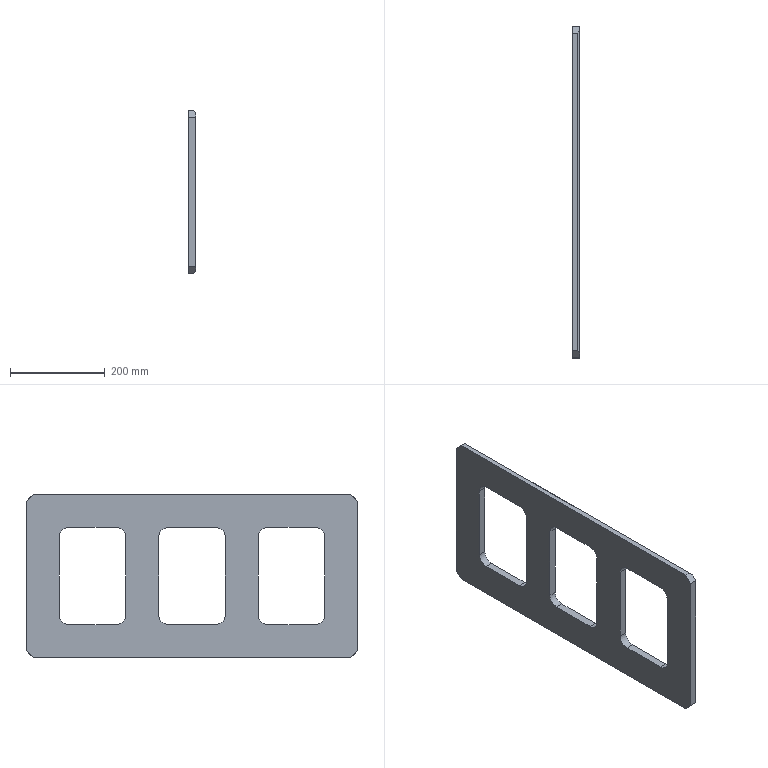Part | SolidWorks | features Chamfer 2, FlatPattern 1, ICE 1, LPattern 1, SMBaseFlange 1, SheetMetal 1 | 1 solid | 36 faces | box 16 x 700 x 345 mm | volume 2478848 mm3 | plane 24 | cylinder 12 | commonest cylinder face diameters 40 x12
STEP:
#1=CARTESIAN_POINT('',(-16.,15.,0.));
#2=VERTEX_POINT('',#1);
#3=CARTESIAN_POINT('',(-5.,15.,0.));
#4=VERTEX_POINT('',#3);
#5=CARTESIAN_POINT('',(-16.,15.,0.));
#6=DIRECTION('',(1.,0.,0.));
#7=VECTOR('',#6,1000.);
#8=LINE('',#5,#7);
#9=EDGE_CURVE('',#2,#4,#8,.T.);
#10=ORIENTED_EDGE('',*,*,#9,.T.);
#11=CARTESIAN_POINT('',(-5.,685.,0.));
#12=VERTEX_POINT('',#11);
#13=CARTESIAN_POINT('',(-5.,685.,0.));
#14=DIRECTION('',(0.,1.,0.));
#15=VECTOR('',#14,1000.);
#16=LINE('',#13,#15);
#17=EDGE_CURVE('',#4,#12,#16,.T.);
#18=ORIENTED_EDGE('',*,*,#17,.T.);
#19=CARTESIAN_POINT('',(-16.,685.,0.));
#20=VERTEX_POINT('',#19);
#21=CARTESIAN_POINT('',(-16.,685.,0.));
#22=DIRECTION('',(-1.,0.,0.));
#23=VECTOR('',#22,1000.);
#24=LINE('',#21,#23);
#25=EDGE_CURVE('',#12,#20,#24,.T.);
#26=ORIENTED_EDGE('',*,*,#25,.T.);
#27=CARTESIAN_POINT('',(-16.,0.,0.));
#28=DIRECTION('',(0.,-1.,0.));
#29=VECTOR('',#28,1000.);
#30=LINE('',#27,#29);
#31=EDGE_CURVE('',#20,#2,#30,.T.);
#32=ORIENTED_EDGE('',*,*,#31,.T.);
#33=EDGE_LOOP('',(#10,#18,#26,#32));
#34=FACE_OUTER_BOUND('',#33,.T.);
#35=CARTESIAN_POINT('',(-16.,0.,0.));
#36=DIRECTION('',(0.,0.,1.));
#37=DIRECTION('',(1.,0.,0.));
#38=AXIS2_PLACEMENT_3D('',#35,#36,#37);
#39=PLANE('',#38);
#40=ADVANCED_FACE('',(#34),#39,.T.);
#41=CARTESIAN_POINT('',(0.,700.,-330.));
#42=VERTEX_POINT('',#41);
#43=CARTESIAN_POINT('',(0.,700.,-15.));
#44=VERTEX_POINT('',#43);
#45=CARTESIAN_POINT('',(0.,700.,0.));
#46=DIRECTION('',(0.,0.,1.));
#47=VECTOR('',#46,1000.);
#48=LINE('',#45,#47);
#49=EDGE_CURVE('',#42,#44,#48,.T.);
#50=ORIENTED_EDGE('',*,*,#49,.F.);
#51=CARTESIAN_POINT('',(-16.,700.,-330.));
#52=VERTEX_POINT('',#51);
#53=CARTESIAN_POINT('',(-16.,700.,-330.));
#54=DIRECTION('',(-1.,0.,0.));
#55=VECTOR('',#54,1000.);
#56=LINE('',#53,#55);
#57=EDGE_CURVE('',#42,#52,#56,.T.);
#58=ORIENTED_EDGE('',*,*,#57,.T.);
#59=CARTESIAN_POINT('',(-16.,700.,-15.));
#60=VERTEX_POINT('',#59);
#61=CARTESIAN_POINT('',(-16.,700.,0.));
#62=DIRECTION('',(0.,0.,1.));
#63=VECTOR('',#62,1000.);
#64=LINE('',#61,#63);
#65=EDGE_CURVE('',#52,#60,#64,.T.);
#66=ORIENTED_EDGE('',*,*,#65,.T.);
#67=CARTESIAN_POINT('',(-16.,700.,-15.));
#68=DIRECTION('',(1.,0.,0.));
#69=VECTOR('',#68,1000.);
#70=LINE('',#67,#69);
#71=EDGE_CURVE('',#60,#44,#70,.T.);
#72=ORIENTED_EDGE('',*,*,#71,.T.);
#73=EDGE_LOOP('',(#50,#58,#66,#72));
#74=FACE_OUTER_BOUND('',#73,.T.);
#75=CARTESIAN_POINT('',(-16.,700.,0.));
#76=DIRECTION('',(0.,1.,0.));
#77=DIRECTION('',(0.,0.,1.));
#78=AXIS2_PLACEMENT_3D('',#75,#76,#77);
#79=PLANE('',#78);
#80=ADVANCED_FACE('',(#74),#79,.T.);
#81=CARTESIAN_POINT('',(-16.,685.,-345.));
#82=VERTEX_POINT('',#81);
#83=CARTESIAN_POINT('',(-5.,685.,-345.));
#84=VERTEX_POINT('',#83);
#85=CARTESIAN_POINT('',(-16.,685.,-345.));
#86=DIRECTION('',(1.,0.,0.));
#87=VECTOR('',#86,1000.);
#88=LINE('',#85,#87);
#89=EDGE_CURVE('',#82,#84,#88,.T.);
#90=ORIENTED_EDGE('',*,*,#89,.T.);
#91=CARTESIAN_POINT('',(-5.,15.,-345.));
#92=VERTEX_POINT('',#91);
#93=CARTESIAN_POINT('',(-5.,15.,-345.));
#94=DIRECTION('',(0.,-1.,0.));
#95=VECTOR('',#94,1000.);
#96=LINE('',#93,#95);
#97=EDGE_CURVE('',#84,#92,#96,.T.);
#98=ORIENTED_EDGE('',*,*,#97,.T.);
#99=CARTESIAN_POINT('',(-16.,15.,-345.));
#100=VERTEX_POINT('',#99);
#101=CARTESIAN_POINT('',(-16.,15.,-345.));
#102=DIRECTION('',(-1.,0.,0.));
#103=VECTOR('',#102,1000.);
#104=LINE('',#101,#103);
#105=EDGE_CURVE('',#92,#100,#104,.T.);
#106=ORIENTED_EDGE('',*,*,#105,.T.);
#107=CARTESIAN_POINT('',(-16.,0.,-345.));
#108=DIRECTION('',(0.,1.,0.));
#109=VECTOR('',#108,1000.);
#110=LINE('',#107,#109);
#111=EDGE_CURVE('',#100,#82,#110,.T.);
#112=ORIENTED_EDGE('',*,*,#111,.T.);
#113=EDGE_LOOP('',(#90,#98,#106,#112));
#114=FACE_OUTER_BOUND('',#113,.T.);
#115=CARTESIAN_POINT('',(-16.,0.,-345.));
#116=DIRECTION('',(0.,0.,-1.));
#117=DIRECTION('',(-1.,0.,0.));
#118=AXIS2_PLACEMENT_3D('',#115,#116,#117);
#119=PLANE('',#118);
#120=ADVANCED_FACE('',(#114),#119,.T.);
#121=CARTESIAN_POINT('',(-16.,0.,-15.));
#122=VERTEX_POINT('',#121);
#123=CARTESIAN_POINT('',(-16.,0.,-330.));
#124=VERTEX_POINT('',#123);
#125=CARTESIAN_POINT('',(-16.,0.,0.));
#126=DIRECTION('',(0.,0.,-1.));
#127=VECTOR('',#126,1000.);
#128=LINE('',#125,#127);
#129=EDGE_CURVE('',#122,#124,#128,.T.);
#130=ORIENTED_EDGE('',*,*,#129,.T.);
#131=CARTESIAN_POINT('',(0.,0.,-330.));
#132=VERTEX_POINT('',#131);
#133=CARTESIAN_POINT('',(-16.,0.,-330.));
#134=DIRECTION('',(1.,0.,0.));
#135=VECTOR('',#134,1000.);
#136=LINE('',#133,#135);
#137=EDGE_CURVE('',#124,#132,#136,.T.);
#138=ORIENTED_EDGE('',*,*,#137,.T.);
#139=CARTESIAN_POINT('',(0.,0.,-15.));
#140=VERTEX_POINT('',#139);
#141=CARTESIAN_POINT('',(0.,0.,0.));
#142=DIRECTION('',(0.,0.,-1.));
#143=VECTOR('',#142,1000.);
#144=LINE('',#141,#143);
#145=EDGE_CURVE('',#140,#132,#144,.T.);
#146=ORIENTED_EDGE('',*,*,#145,.F.);
#147=CARTESIAN_POINT('',(-16.,0.,-15.));
#148=DIRECTION('',(-1.,0.,0.));
#149=VECTOR('',#148,1000.);
#150=LINE('',#147,#149);
#151=EDGE_CURVE('',#140,#122,#150,.T.);
#152=ORIENTED_EDGE('',*,*,#151,.T.);
#153=EDGE_LOOP('',(#130,#138,#146,#152));
#154=FACE_OUTER_BOUND('',#153,.T.);
#155=CARTESIAN_POINT('',(-16.,0.,0.));
#156=DIRECTION('',(0.,-1.,0.));
#157=DIRECTION('',(0.,0.,-1.));
#158=AXIS2_PLACEMENT_3D('',#155,#156,#157);
#159=PLANE('',#158);
#160=ADVANCED_FACE('',(#154),#159,.T.);
#161=CARTESIAN_POINT('',(-16.,300.,-70.));
#162=VERTEX_POINT('',#161);
#163=CARTESIAN_POINT('',(-16.,280.,-90.));
#164=VERTEX_POINT('',#163);
#165=CARTESIAN_POINT('',(-16.,300.,-90.));
#166=DIRECTION('',(1.,0.,0.));
#167=DIRECTION('',(0.,0.,1.));
#168=AXIS2_PLACEMENT_3D('',#165,#166,#167);
#169=CIRCLE('',#168,20.);
#170=EDGE_CURVE('',#162,#164,#169,.T.);
#171=ORIENTED_EDGE('',*,*,#170,.T.);
#172=CARTESIAN_POINT('',(-16.,280.,-255.));
#173=VERTEX_POINT('',#172);
#174=CARTESIAN_POINT('',(-16.,280.,-90.));
#175=DIRECTION('',(0.,0.,-1.));
#176=VECTOR('',#175,1000.);
#177=LINE('',#174,#176);
#178=EDGE_CURVE('',#164,#173,#177,.T.);
#179=ORIENTED_EDGE('',*,*,#178,.T.);
#180=CARTESIAN_POINT('',(-16.,300.,-275.));
#181=VERTEX_POINT('',#180);
#182=CARTESIAN_POINT('',(-16.,300.,-255.));
#183=DIRECTION('',(1.,0.,0.));
#184=DIRECTION('',(0.,0.,-1.));
#185=AXIS2_PLACEMENT_3D('',#182,#183,#184);
#186=CIRCLE('',#185,20.);
#187=EDGE_CURVE('',#173,#181,#186,.T.);
#188=ORIENTED_EDGE('',*,*,#187,.T.);
#189=CARTESIAN_POINT('',(-16.,400.,-275.));
#190=VERTEX_POINT('',#189);
#191=CARTESIAN_POINT('',(-16.,400.,-275.));
#192=DIRECTION('',(0.,1.,0.));
#193=VECTOR('',#192,1000.);
#194=LINE('',#191,#193);
#195=EDGE_CURVE('',#181,#190,#194,.T.);
#196=ORIENTED_EDGE('',*,*,#195,.T.);
#197=CARTESIAN_POINT('',(-16.,420.,-255.));
#198=VERTEX_POINT('',#197);
#199=CARTESIAN_POINT('',(-16.,400.,-255.));
#200=DIRECTION('',(1.,0.,0.));
#201=DIRECTION('',(0.,0.,-1.));
#202=AXIS2_PLACEMENT_3D('',#199,#200,#201);
#203=CIRCLE('',#202,20.);
#204=EDGE_CURVE('',#190,#198,#203,.T.);
#205=ORIENTED_EDGE('',*,*,#204,.T.);
#206=CARTESIAN_POINT('',(-16.,420.,-90.));
#207=VERTEX_POINT('',#206);
#208=CARTESIAN_POINT('',(-16.,420.,-90.));
#209=DIRECTION('',(0.,0.,1.));
#210=VECTOR('',#209,1000.);
#211=LINE('',#208,#210);
#212=EDGE_CURVE('',#198,#207,#211,.T.);
#213=ORIENTED_EDGE('',*,*,#212,.T.);
#214=CARTESIAN_POINT('',(-16.,400.,-70.));
#215=VERTEX_POINT('',#214);
#216=CARTESIAN_POINT('',(-16.,400.,-90.));
#217=DIRECTION('',(1.,0.,0.));
#218=DIRECTION('',(0.,0.,-1.));
#219=AXIS2_PLACEMENT_3D('',#216,#217,#218);
#220=CIRCLE('',#219,20.);
#221=EDGE_CURVE('',#207,#215,#220,.T.);
#222=ORIENTED_EDGE('',*,*,#221,.T.);
#223=CARTESIAN_POINT('',(-16.,400.,-70.));
#224=DIRECTION('',(0.,-1.,0.));
#225=VECTOR('',#224,1000.);
#226=LINE('',#223,#225);
#227=EDGE_CURVE('',#215,#162,#226,.T.);
#228=ORIENTED_EDGE('',*,*,#227,.T.);
#229=EDGE_LOOP('',(#171,#179,#188,#196,#205,#213,#222,#228));
#230=FACE_BOUND('',#229,.T.);
#231=CARTESIAN_POINT('',(-16.,510.,-70.));
#232=VERTEX_POINT('',#231);
#233=CARTESIAN_POINT('',(-16.,490.,-90.));
#234=VERTEX_POINT('',#233);
#235=CARTESIAN_POINT('',(-16.,510.,-90.));
#236=DIRECTION('',(1.,0.,0.));
#237=DIRECTION('',(0.,0.,1.));
#238=AXIS2_PLACEMENT_3D('',#235,#236,#237);
#239=CIRCLE('',#238,20.);
#240=EDGE_CURVE('',#232,#234,#239,.T.);
#241=ORIENTED_EDGE('',*,*,#240,.T.);
#242=CARTESIAN_POINT('',(-16.,490.,-255.));
#243=VERTEX_POINT('',#242);
#244=CARTESIAN_POINT('',(-16.,490.,-90.));
#245=DIRECTION('',(0.,0.,-1.));
#246=VECTOR('',#245,1000.);
#247=LINE('',#244,#246);
#248=EDGE_CURVE('',#234,#243,#247,.T.);
#249=ORIENTED_EDGE('',*,*,#248,.T.);
#250=CARTESIAN_POINT('',(-16.,510.,-275.));
#251=VERTEX_POINT('',#250);
#252=CARTESIAN_POINT('',(-16.,510.,-255.));
#253=DIRECTION('',(1.,0.,0.));
#254=DIRECTION('',(0.,0.,-1.));
#255=AXIS2_PLACEMENT_3D('',#252,#253,#254);
#256=CIRCLE('',#255,20.);
#257=EDGE_CURVE('',#243,#251,#256,.T.);
#258=ORIENTED_EDGE('',*,*,#257,.T.);
#259=CARTESIAN_POINT('',(-16.,610.,-275.));
#260=VERTEX_POINT('',#259);
#261=CARTESIAN_POINT('',(-16.,610.,-275.));
#262=DIRECTION('',(0.,1.,0.));
#263=VECTOR('',#262,1000.);
#264=LINE('',#261,#263);
#265=EDGE_CURVE('',#251,#260,#264,.T.);
#266=ORIENTED_EDGE('',*,*,#265,.T.);
#267=CARTESIAN_POINT('',(-16.,630.,-255.));
#268=VERTEX_POINT('',#267);
#269=CARTESIAN_POINT('',(-16.,610.,-255.));
#270=DIRECTION('',(1.,0.,0.));
#271=DIRECTION('',(0.,0.,-1.));
#272=AXIS2_PLACEMENT_3D('',#269,#270,#271);
#273=CIRCLE('',#272,20.);
#274=EDGE_CURVE('',#260,#268,#273,.T.);
#275=ORIENTED_EDGE('',*,*,#274,.T.);
#276=CARTESIAN_POINT('',(-16.,630.,-90.));
#277=VERTEX_POINT('',#276);
#278=CARTESIAN_POINT('',(-16.,630.,-90.));
#279=DIRECTION('',(0.,0.,1.));
#280=VECTOR('',#279,1000.);
#281=LINE('',#278,#280);
#282=EDGE_CURVE('',#268,#277,#281,.T.);
#283=ORIENTED_EDGE('',*,*,#282,.T.);
#284=CARTESIAN_POINT('',(-16.,610.,-70.));
#285=VERTEX_POINT('',#284);
#286=CARTESIAN_POINT('',(-16.,610.,-90.));
#287=DIRECTION('',(1.,0.,0.));
#288=DIRECTION('',(0.,0.,-1.));
#289=AXIS2_PLACEMENT_3D('',#286,#287,#288);
#290=CIRCLE('',#289,20.);
#291=EDGE_CURVE('',#277,#285,#290,.T.);
#292=ORIENTED_EDGE('',*,*,#291,.T.);
#293=CARTESIAN_POINT('',(-16.,610.,-70.));
#294=DIRECTION('',(0.,-1.,0.));
#295=VECTOR('',#294,1000.);
#296=LINE('',#293,#295);
#297=EDGE_CURVE('',#285,#232,#296,.T.);
#298=ORIENTED_EDGE('',*,*,#297,.T.);
#299=EDGE_LOOP('',(#241,#249,#258,#266,#275,#283,#292,#298));
#300=FACE_BOUND('',#299,.T.);
#301=ORIENTED_EDGE('',*,*,#111,.F.);
#302=CARTESIAN_POINT('',(-16.,185.,-515.));
#303=DIRECTION('',(0.,-0.7071,0.7071));
#304=VECTOR('',#303,1000.);
#305=LINE('',#302,#304);
#306=EDGE_CURVE('',#100,#124,#305,.T.);
#307=ORIENTED_EDGE('',*,*,#306,.T.);
#308=ORIENTED_EDGE('',*,*,#129,.F.);
#309=CARTESIAN_POINT('',(-16.,357.5,342.5));
#310=DIRECTION('',(0.,0.7071,0.7071));
#311=VECTOR('',#310,1000.);
#312=LINE('',#309,#311);
#313=EDGE_CURVE('',#122,#2,#312,.T.);
#314=ORIENTED_EDGE('',*,*,#313,.T.);
#315=ORIENTED_EDGE('',*,*,#31,.F.);
#316=CARTESIAN_POINT('',(-16.,692.5,-7.5));
#317=DIRECTION('',(0.,0.7071,-0.7071));
#318=VECTOR('',#317,1000.);
#319=LINE('',#316,#318);
#320=EDGE_CURVE('',#20,#60,#319,.T.);
#321=ORIENTED_EDGE('',*,*,#320,.T.);
#322=ORIENTED_EDGE('',*,*,#65,.F.);
#323=CARTESIAN_POINT('',(-16.,865.,-165.));
#324=DIRECTION('',(0.,-0.7071,-0.7071));
#325=VECTOR('',#324,1000.);
#326=LINE('',#323,#325);
#327=EDGE_CURVE('',#52,#82,#326,.T.);
#328=ORIENTED_EDGE('',*,*,#327,.T.);
#329=EDGE_LOOP('',(#301,#307,#308,#314,#315,#321,#322,#328));
#330=FACE_OUTER_BOUND('',#329,.T.);
#331=CARTESIAN_POINT('',(-16.,90.,-70.));
#332=VERTEX_POINT('',#331);
#333=CARTESIAN_POINT('',(-16.,70.,-90.));
#334=VERTEX_POINT('',#333);
#335=CARTESIAN_POINT('',(-16.,90.,-90.));
#336=DIRECTION('',(1.,0.,0.));
#337=DIRECTION('',(0.,0.,1.));
#338=AXIS2_PLACEMENT_3D('',#335,#336,#337);
#339=CIRCLE('',#338,20.);
#340=EDGE_CURVE('',#332,#334,#339,.T.);
#341=ORIENTED_EDGE('',*,*,#340,.T.);
#342=CARTESIAN_POINT('',(-16.,70.,-255.));
#343=VERTEX_POINT('',#342);
#344=CARTESIAN_POINT('',(-16.,70.,-90.));
#345=DIRECTION('',(0.,0.,-1.));
#346=VECTOR('',#345,1000.);
#347=LINE('',#344,#346);
#348=EDGE_CURVE('',#334,#343,#347,.T.);
#349=ORIENTED_EDGE('',*,*,#348,.T.);
#350=CARTESIAN_POINT('',(-16.,90.,-275.));
#351=VERTEX_POINT('',#350);
#352=CARTESIAN_POINT('',(-16.,90.,-255.));
#353=DIRECTION('',(1.,0.,0.));
#354=DIRECTION('',(0.,0.,-1.));
#355=AXIS2_PLACEMENT_3D('',#352,#353,#354);
#356=CIRCLE('',#355,20.);
#357=EDGE_CURVE('',#343,#351,#356,.T.);
#358=ORIENTED_EDGE('',*,*,#357,.T.);
#359=CARTESIAN_POINT('',(-16.,190.,-275.));
#360=VERTEX_POINT('',#359);
#361=CARTESIAN_POINT('',(-16.,190.,-275.));
#362=DIRECTION('',(0.,1.,0.));
#363=VECTOR('',#362,1000.);
#364=LINE('',#361,#363);
#365=EDGE_CURVE('',#351,#360,#364,.T.);
#366=ORIENTED_EDGE('',*,*,#365,.T.);
#367=CARTESIAN_POINT('',(-16.,210.,-255.));
#368=VERTEX_POINT('',#367);
#369=CARTESIAN_POINT('',(-16.,190.,-255.));
#370=DIRECTION('',(1.,0.,0.));
#371=DIRECTION('',(0.,0.,-1.));
#372=AXIS2_PLACEMENT_3D('',#369,#370,#371);
#373=CIRCLE('',#372,20.);
#374=EDGE_CURVE('',#360,#368,#373,.T.);
#375=ORIENTED_EDGE('',*,*,#374,.T.);
#376=CARTESIAN_POINT('',(-16.,210.,-90.));
#377=VERTEX_POINT('',#376);
#378=CARTESIAN_POINT('',(-16.,210.,-90.));
#379=DIRECTION('',(0.,0.,1.));
#380=VECTOR('',#379,1000.);
#381=LINE('',#378,#380);
#382=EDGE_CURVE('',#368,#377,#381,.T.);
#383=ORIENTED_EDGE('',*,*,#382,.T.);
#384=CARTESIAN_POINT('',(-16.,190.,-70.));
#385=VERTEX_POINT('',#384);
#386=CARTESIAN_POINT('',(-16.,190.,-90.));
#387=DIRECTION('',(1.,0.,0.));
#388=DIRECTION('',(0.,0.,-1.));
#389=AXIS2_PLACEMENT_3D('',#386,#387,#388);
#390=CIRCLE('',#389,20.);
#391=EDGE_CURVE('',#377,#385,#390,.T.);
#392=ORIENTED_EDGE('',*,*,#391,.T.);
#393=CARTESIAN_POINT('',(-16.,190.,-70.));
#394=DIRECTION('',(0.,-1.,0.));
#395=VECTOR('',#394,1000.);
#396=LINE('',#393,#395);
#397=EDGE_CURVE('',#385,#332,#396,.T.);
#398=ORIENTED_EDGE('',*,*,#397,.T.);
#399=EDGE_LOOP('',(#341,#349,#358,#366,#375,#383,#392,#398));
#400=FACE_BOUND('',#399,.T.);
#401=CARTESIAN_POINT('',(-16.,700.,0.));
#402=DIRECTION('',(-1.,0.,0.));
#403=DIRECTION('',(0.,0.,1.));
#404=AXIS2_PLACEMENT_3D('',#401,#402,#403);
#405=PLANE('',#404);
#406=ADVANCED_FACE('',(#230,#300,#330,#400),#405,.T.);
#407=CARTESIAN_POINT('',(0.,280.,-90.));
#408=VERTEX_POINT('',#407);
#409=CARTESIAN_POINT('',(0.,280.,-255.));
#410=VERTEX_POINT('',#409);
#411=CARTESIAN_POINT('',(0.,280.,-90.));
#412=DIRECTION('',(0.,0.,-1.));
#413=VECTOR('',#412,1000.);
#414=LINE('',#411,#413);
#415=EDGE_CURVE('',#408,#410,#414,.T.);
#416=ORIENTED_EDGE('',*,*,#415,.F.);
#417=CARTESIAN_POINT('',(0.,300.,-70.));
#418=VERTEX_POINT('',#417);
#419=CARTESIAN_POINT('',(0.,300.,-90.));
#420=DIRECTION('',(1.,0.,0.));
#421=DIRECTION('',(0.,0.,1.));
#422=AXIS2_PLACEMENT_3D('',#419,#420,#421);
#423=CIRCLE('',#422,20.);
#424=EDGE_CURVE('',#418,#408,#423,.T.);
#425=ORIENTED_EDGE('',*,*,#424,.F.);
#426=CARTESIAN_POINT('',(0.,400.,-70.));
#427=VERTEX_POINT('',#426);
#428=CARTESIAN_POINT('',(0.,400.,-70.));
#429=DIRECTION('',(0.,-1.,0.));
#430=VECTOR('',#429,1000.);
#431=LINE('',#428,#430);
#432=EDGE_CURVE('',#427,#418,#431,.T.);
#433=ORIENTED_EDGE('',*,*,#432,.F.);
#434=CARTESIAN_POINT('',(0.,420.,-90.));
#435=VERTEX_POINT('',#434);
#436=CARTESIAN_POINT('',(0.,400.,-90.));
#437=DIRECTION('',(1.,0.,0.));
#438=DIRECTION('',(0.,0.,-1.));
#439=AXIS2_PLACEMENT_3D('',#436,#437,#438);
#440=CIRCLE('',#439,20.);
#441=EDGE_CURVE('',#435,#427,#440,.T.);
#442=ORIENTED_EDGE('',*,*,#441,.F.);
#443=CARTESIAN_POINT('',(0.,420.,-255.));
#444=VERTEX_POINT('',#443);
#445=CARTESIAN_POINT('',(0.,420.,-90.));
#446=DIRECTION('',(0.,0.,1.));
#447=VECTOR('',#446,1000.);
#448=LINE('',#445,#447);
#449=EDGE_CURVE('',#444,#435,#448,.T.);
#450=ORIENTED_EDGE('',*,*,#449,.F.);
#451=CARTESIAN_POINT('',(0.,400.,-275.));
#452=VERTEX_POINT('',#451);
#453=CARTESIAN_POINT('',(0.,400.,-255.));
#454=DIRECTION('',(1.,0.,0.));
#455=DIRECTION('',(0.,0.,-1.));
#456=AXIS2_PLACEMENT_3D('',#453,#454,#455);
#457=CIRCLE('',#456,20.);
#458=EDGE_CURVE('',#452,#444,#457,.T.);
#459=ORIENTED_EDGE('',*,*,#458,.F.);
#460=CARTESIAN_POINT('',(0.,300.,-275.));
#461=VERTEX_POINT('',#460);
#462=CARTESIAN_POINT('',(0.,400.,-275.));
#463=DIRECTION('',(0.,1.,0.));
#464=VECTOR('',#463,1000.);
#465=LINE('',#462,#464);
#466=EDGE_CURVE('',#461,#452,#465,.T.);
#467=ORIENTED_EDGE('',*,*,#466,.F.);
#468=CARTESIAN_POINT('',(0.,300.,-255.));
#469=DIRECTION('',(1.,0.,0.));
#470=DIRECTION('',(0.,0.,-1.));
#471=AXIS2_PLACEMENT_3D('',#468,#469,#470);
#472=CIRCLE('',#471,20.);
#473=EDGE_CURVE('',#410,#461,#472,.T.);
#474=ORIENTED_EDGE('',*,*,#473,.F.);
#475=EDGE_LOOP('',(#416,#425,#433,#442,#450,#459,#467,#474));
#476=FACE_BOUND('',#475,.T.);
#477=CARTESIAN_POINT('',(0.,490.,-90.));
#478=VERTEX_POINT('',#477);
#479=CARTESIAN_POINT('',(0.,490.,-255.));
#480=VERTEX_POINT('',#479);
#481=CARTESIAN_POINT('',(0.,490.,-90.));
#482=DIRECTION('',(0.,0.,-1.));
#483=VECTOR('',#482,1000.);
#484=LINE('',#481,#483);
#485=EDGE_CURVE('',#478,#480,#484,.T.);
#486=ORIENTED_EDGE('',*,*,#485,.F.);
#487=CARTESIAN_POINT('',(0.,510.,-70.));
#488=VERTEX_POINT('',#487);
#489=CARTESIAN_POINT('',(0.,510.,-90.));
#490=DIRECTION('',(1.,0.,0.));
#491=DIRECTION('',(0.,0.,1.));
#492=AXIS2_PLACEMENT_3D('',#489,#490,#491);
#493=CIRCLE('',#492,20.);
#494=EDGE_CURVE('',#488,#478,#493,.T.);
#495=ORIENTED_EDGE('',*,*,#494,.F.);
#496=CARTESIAN_POINT('',(0.,610.,-70.));
#497=VERTEX_POINT('',#496);
#498=CARTESIAN_POINT('',(0.,610.,-70.));
#499=DIRECTION('',(0.,-1.,0.));
#500=VECTOR('',#499,1000.);
#501=LINE('',#498,#500);
#502=EDGE_CURVE('',#497,#488,#501,.T.);
#503=ORIENTED_EDGE('',*,*,#502,.F.);
#504=CARTESIAN_POINT('',(0.,630.,-90.));
#505=VERTEX_POINT('',#504);
#506=CARTESIAN_POINT('',(0.,610.,-90.));
#507=DIRECTION('',(1.,0.,0.));
#508=DIRECTION('',(0.,0.,-1.));
#509=AXIS2_PLACEMENT_3D('',#506,#507,#508);
#510=CIRCLE('',#509,20.);
#511=EDGE_CURVE('',#505,#497,#510,.T.);
#512=ORIENTED_EDGE('',*,*,#511,.F.);
#513=CARTESIAN_POINT('',(0.,630.,-255.));
#514=VERTEX_POINT('',#513);
#515=CARTESIAN_POINT('',(0.,630.,-90.));
#516=DIRECTION('',(0.,0.,1.));
#517=VECTOR('',#516,1000.);
#518=LINE('',#515,#517);
#519=EDGE_CURVE('',#514,#505,#518,.T.);
#520=ORIENTED_EDGE('',*,*,#519,.F.);
#521=CARTESIAN_POINT('',(0.,610.,-275.));
#522=VERTEX_POINT('',#521);
#523=CARTESIAN_POINT('',(0.,610.,-255.));
#524=DIRECTION('',(1.,0.,0.));
#525=DIRECTION('',(0.,0.,-1.));
#526=AXIS2_PLACEMENT_3D('',#523,#524,#525);
#527=CIRCLE('',#526,20.);
#528=EDGE_CURVE('',#522,#514,#527,.T.);
#529=ORIENTED_EDGE('',*,*,#528,.F.);
#530=CARTESIAN_POINT('',(0.,510.,-275.));
#531=VERTEX_POINT('',#530);
#532=CARTESIAN_POINT('',(0.,610.,-275.));
#533=DIRECTION('',(0.,1.,0.));
#534=VECTOR('',#533,1000.);
#535=LINE('',#532,#534);
#536=EDGE_CURVE('',#531,#522,#535,.T.);
#537=ORIENTED_EDGE('',*,*,#536,.F.);
#538=CARTESIAN_POINT('',(0.,510.,-255.));
#539=DIRECTION('',(1.,0.,0.));
#540=DIRECTION('',(0.,0.,-1.));
#541=AXIS2_PLACEMENT_3D('',#538,#539,#540);
#542=CIRCLE('',#541,20.);
#543=EDGE_CURVE('',#480,#531,#542,.T.);
#544=ORIENTED_EDGE('',*,*,#543,.F.);
#545=EDGE_LOOP('',(#486,#495,#503,#512,#520,#529,#537,#544));
#546=FACE_BOUND('',#545,.T.);
#547=CARTESIAN_POINT('',(0.,10.,-340.));
#548=VERTEX_POINT('',#547);
#549=CARTESIAN_POINT('',(0.,0.,-330.));
#550=DIRECTION('',(0.,0.7071,-0.7071));
#551=VECTOR('',#550,1000.);
#552=LINE('',#549,#551);
#553=EDGE_CURVE('',#132,#548,#552,.T.);
#554=ORIENTED_EDGE('',*,*,#553,.T.);
#555=CARTESIAN_POINT('',(0.,690.,-340.));
#556=VERTEX_POINT('',#555);
#557=CARTESIAN_POINT('',(0.,685.,-340.));
#558=DIRECTION('',(0.,1.,0.));
#559=VECTOR('',#558,1000.);
#560=LINE('',#557,#559);
#561=EDGE_CURVE('',#548,#556,#560,.T.);
#562=ORIENTED_EDGE('',*,*,#561,.T.);
#563=CARTESIAN_POINT('',(0.,685.,-345.));
#564=DIRECTION('',(0.,0.7071,0.7071));
#565=VECTOR('',#564,1000.);
#566=LINE('',#563,#565);
#567=EDGE_CURVE('',#556,#42,#566,.T.);
#568=ORIENTED_EDGE('',*,*,#567,.T.);
#569=ORIENTED_EDGE('',*,*,#49,.T.);
#570=CARTESIAN_POINT('',(0.,690.,-5.));
#571=VERTEX_POINT('',#570);
#572=CARTESIAN_POINT('',(0.,700.,-15.));
#573=DIRECTION('',(0.,-0.7071,0.7071));
#574=VECTOR('',#573,1000.);
#575=LINE('',#572,#574);
#576=EDGE_CURVE('',#44,#571,#575,.T.);
#577=ORIENTED_EDGE('',*,*,#576,.T.);
#578=CARTESIAN_POINT('',(0.,10.,-5.));
#579=VERTEX_POINT('',#578);
#580=CARTESIAN_POINT('',(0.,15.,-5.));
#581=DIRECTION('',(0.,-1.,0.));
#582=VECTOR('',#581,1000.);
#583=LINE('',#580,#582);
#584=EDGE_CURVE('',#571,#579,#583,.T.);
#585=ORIENTED_EDGE('',*,*,#584,.T.);
#586=CARTESIAN_POINT('',(0.,15.,0.));
#587=DIRECTION('',(0.,-0.7071,-0.7071));
#588=VECTOR('',#587,1000.);
#589=LINE('',#586,#588);
#590=EDGE_CURVE('',#579,#140,#589,.T.);
#591=ORIENTED_EDGE('',*,*,#590,.T.);
#592=ORIENTED_EDGE('',*,*,#145,.T.);
#593=EDGE_LOOP('',(#554,#562,#568,#569,#577,#585,#591,#592));
#594=FACE_OUTER_BOUND('',#593,.T.);
#595=CARTESIAN_POINT('',(0.,90.,-70.));
#596=VERTEX_POINT('',#595);
#597=CARTESIAN_POINT('',(0.,70.,-90.));
#598=VERTEX_POINT('',#597);
#599=CARTESIAN_POINT('',(0.,90.,-90.));
#600=DIRECTION('',(1.,0.,0.));
#601=DIRECTION('',(0.,0.,1.));
#602=AXIS2_PLACEMENT_3D('',#599,#600,#601);
#603=CIRCLE('',#602,20.);
#604=EDGE_CURVE('',#596,#598,#603,.T.);
#605=ORIENTED_EDGE('',*,*,#604,.F.);
#606=CARTESIAN_POINT('',(0.,190.,-70.));
#607=VERTEX_POINT('',#606);
#608=CARTESIAN_POINT('',(0.,190.,-70.));
#609=DIRECTION('',(0.,-1.,0.));
#610=VECTOR('',#609,1000.);
#611=LINE('',#608,#610);
#612=EDGE_CURVE('',#607,#596,#611,.T.);
#613=ORIENTED_EDGE('',*,*,#612,.F.);
#614=CARTESIAN_POINT('',(0.,210.,-90.));
#615=VERTEX_POINT('',#614);
#616=CARTESIAN_POINT('',(0.,190.,-90.));
#617=DIRECTION('',(1.,0.,0.));
#618=DIRECTION('',(0.,0.,-1.));
#619=AXIS2_PLACEMENT_3D('',#616,#617,#618);
#620=CIRCLE('',#619,20.);
#621=EDGE_CURVE('',#615,#607,#620,.T.);
#622=ORIENTED_EDGE('',*,*,#621,.F.);
#623=CARTESIAN_POINT('',(0.,210.,-255.));
#624=VERTEX_POINT('',#623);
#625=CARTESIAN_POINT('',(0.,210.,-90.));
#626=DIRECTION('',(0.,0.,1.));
#627=VECTOR('',#626,1000.);
#628=LINE('',#625,#627);
#629=EDGE_CURVE('',#624,#615,#628,.T.);
#630=ORIENTED_EDGE('',*,*,#629,.F.);
#631=CARTESIAN_POINT('',(0.,190.,-275.));
#632=VERTEX_POINT('',#631);
#633=CARTESIAN_POINT('',(0.,190.,-255.));
#634=DIRECTION('',(1.,0.,0.));
#635=DIRECTION('',(0.,0.,-1.));
#636=AXIS2_PLACEMENT_3D('',#633,#634,#635);
#637=CIRCLE('',#636,20.);
#638=EDGE_CURVE('',#632,#624,#637,.T.);
#639=ORIENTED_EDGE('',*,*,#638,.F.);
#640=CARTESIAN_POINT('',(0.,90.,-275.));
#641=VERTEX_POINT('',#640);
#642=CARTESIAN_POINT('',(0.,190.,-275.));
#643=DIRECTION('',(0.,1.,0.));
#644=VECTOR('',#643,1000.);
#645=LINE('',#642,#644);
#646=EDGE_CURVE('',#641,#632,#645,.T.);
#647=ORIENTED_EDGE('',*,*,#646,.F.);
#648=CARTESIAN_POINT('',(0.,70.,-255.));
#649=VERTEX_POINT('',#648);
#650=CARTESIAN_POINT('',(0.,90.,-255.));
#651=DIRECTION('',(1.,0.,0.));
#652=DIRECTION('',(0.,0.,-1.));
#653=AXIS2_PLACEMENT_3D('',#650,#651,#652);
#654=CIRCLE('',#653,20.);
#655=EDGE_CURVE('',#649,#641,#654,.T.);
#656=ORIENTED_EDGE('',*,*,#655,.F.);
#657=CARTESIAN_POINT('',(0.,70.,-90.));
#658=DIRECTION('',(0.,0.,-1.));
#659=VECTOR('',#658,1000.);
#660=LINE('',#657,#659);
#661=EDGE_CURVE('',#598,#649,#660,.T.);
#662=ORIENTED_EDGE('',*,*,#661,.F.);
#663=EDGE_LOOP('',(#605,#613,#622,#630,#639,#647,#656,#662));
#664=FACE_BOUND('',#663,.T.);
#665=CARTESIAN_POINT('',(0.,700.,0.));
#666=DIRECTION('',(-1.,0.,0.));
#667=DIRECTION('',(0.,0.,1.));
#668=AXIS2_PLACEMENT_3D('',#665,#666,#667);
#669=PLANE('',#668);
#670=ADVANCED_FACE('',(#476,#546,#594,#664),#669,.F.);
#671=ORIENTED_EDGE('',*,*,#105,.F.);
#672=CARTESIAN_POINT('',(1.333,8.667,-338.667));
#673=DIRECTION('',(0.5774,-0.5774,0.5774));
#674=VECTOR('',#673,1000.);
#675=LINE('',#672,#674);
#676=EDGE_CURVE('',#92,#548,#675,.T.);
#677=ORIENTED_EDGE('',*,*,#676,.T.);
#678=ORIENTED_EDGE('',*,*,#553,.F.);
#679=ORIENTED_EDGE('',*,*,#137,.F.);
#680=ORIENTED_EDGE('',*,*,#306,.F.);
#681=EDGE_LOOP('',(#671,#677,#678,#679,#680));
#682=FACE_OUTER_BOUND('',#681,.T.);
#683=CARTESIAN_POINT('',(-16.,0.,-330.));
#684=DIRECTION('',(0.,0.7071,0.7071));
#685=DIRECTION('',(0.,-0.7071,0.7071));
#686=AXIS2_PLACEMENT_3D('',#683,#684,#685);
#687=PLANE('',#686);
#688=ADVANCED_FACE('',(#682),#687,.F.);
#689=ORIENTED_EDGE('',*,*,#567,.F.);
#690=CARTESIAN_POINT('',(-8.667,681.333,-348.667));
#691=DIRECTION('',(-0.5774,-0.5774,-0.5774));
#692=VECTOR('',#691,1000.);
#693=LINE('',#690,#692);
#694=EDGE_CURVE('',#556,#84,#693,.T.);
#695=ORIENTED_EDGE('',*,*,#694,.T.);
#696=ORIENTED_EDGE('',*,*,#89,.F.);
#697=ORIENTED_EDGE('',*,*,#327,.F.);
#698=ORIENTED_EDGE('',*,*,#57,.F.);
#699=EDGE_LOOP('',(#689,#695,#696,#697,#698));
#700=FACE_OUTER_BOUND('',#699,.T.);
#701=CARTESIAN_POINT('',(-16.,685.,-345.));
#702=DIRECTION('',(0.,-0.7071,0.7071));
#703=DIRECTION('',(0.,-0.7071,-0.7071));
#704=AXIS2_PLACEMENT_3D('',#701,#702,#703);
#705=PLANE('',#704);
#706=ADVANCED_FACE('',(#700),#705,.F.);
#707=ORIENTED_EDGE('',*,*,#590,.F.);
#708=CARTESIAN_POINT('',(-8.667,18.667,3.667));
#709=DIRECTION('',(-0.5774,0.5774,0.5774));
#710=VECTOR('',#709,1000.);
#711=LINE('',#708,#710);
#712=EDGE_CURVE('',#579,#4,#711,.T.);
#713=ORIENTED_EDGE('',*,*,#712,.T.);
#714=ORIENTED_EDGE('',*,*,#9,.F.);
#715=ORIENTED_EDGE('',*,*,#313,.F.);
#716=ORIENTED_EDGE('',*,*,#151,.F.);
#717=EDGE_LOOP('',(#707,#713,#714,#715,#716));
#718=FACE_OUTER_BOUND('',#717,.T.);
#719=CARTESIAN_POINT('',(-16.,15.,0.));
#720=DIRECTION('',(0.,0.7071,-0.7071));
#721=DIRECTION('',(0.,0.7071,0.7071));
#722=AXIS2_PLACEMENT_3D('',#719,#720,#721);
#723=PLANE('',#722);
#724=ADVANCED_FACE('',(#718),#723,.F.);
#725=ORIENTED_EDGE('',*,*,#25,.F.);
#726=CARTESIAN_POINT('',(1.333,691.333,-6.333));
#727=DIRECTION('',(0.5774,0.5774,-0.5774));
#728=VECTOR('',#727,1000.);
#729=LINE('',#726,#728);
#730=EDGE_CURVE('',#12,#571,#729,.T.);
#731=ORIENTED_EDGE('',*,*,#730,.T.);
#732=ORIENTED_EDGE('',*,*,#576,.F.);
#733=ORIENTED_EDGE('',*,*,#71,.F.);
#734=ORIENTED_EDGE('',*,*,#320,.F.);
#735=EDGE_LOOP('',(#725,#731,#732,#733,#734));
#736=FACE_OUTER_BOUND('',#735,.T.);
#737=CARTESIAN_POINT('',(-16.,700.,-15.));
#738=DIRECTION('',(0.,-0.7071,-0.7071));
#739=DIRECTION('',(0.,0.7071,-0.7071));
#740=AXIS2_PLACEMENT_3D('',#737,#738,#739);
#741=PLANE('',#740);
#742=ADVANCED_FACE('',(#736),#741,.F.);
#743=ORIENTED_EDGE('',*,*,#494,.T.);
#744=CARTESIAN_POINT('',(-16.,490.,-90.));
#745=DIRECTION('',(1.,0.,0.));
#746=VECTOR('',#745,1000.);
#747=LINE('',#744,#746);
#748=EDGE_CURVE('',#234,#478,#747,.T.);
#749=ORIENTED_EDGE('',*,*,#748,.F.);
#750=ORIENTED_EDGE('',*,*,#240,.F.);
#751=CARTESIAN_POINT('',(-16.,510.,-70.));
#752=DIRECTION('',(1.,0.,0.));
#753=VECTOR('',#752,1000.);
#754=LINE('',#751,#753);
#755=EDGE_CURVE('',#232,#488,#754,.T.);
#756=ORIENTED_EDGE('',*,*,#755,.T.);
#757=EDGE_LOOP('',(#743,#749,#750,#756));
#758=FACE_OUTER_BOUND('',#757,.T.);
#759=CARTESIAN_POINT('',(-16.,510.,-90.));
#760=DIRECTION('',(1.,0.,0.));
#761=DIRECTION('',(0.,0.,-1.));
#762=AXIS2_PLACEMENT_3D('',#759,#760,#761);
#763=CYLINDRICAL_SURFACE('',#762,20.);
#764=ADVANCED_FACE('',(#758),#763,.F.);
#765=ORIENTED_EDGE('',*,*,#502,.T.);
#766=ORIENTED_EDGE('',*,*,#755,.F.);
#767=ORIENTED_EDGE('',*,*,#297,.F.);
#768=CARTESIAN_POINT('',(-16.,610.,-70.));
#769=DIRECTION('',(1.,0.,0.));
#770=VECTOR('',#769,1000.);
#771=LINE('',#768,#770);
#772=EDGE_CURVE('',#285,#497,#771,.T.);
#773=ORIENTED_EDGE('',*,*,#772,.T.);
#774=EDGE_LOOP('',(#765,#766,#767,#773));
#775=FACE_OUTER_BOUND('',#774,.T.);
#776=CARTESIAN_POINT('',(-16.,610.,-70.));
#777=DIRECTION('',(0.,0.,1.));
#778=DIRECTION('',(0.,-1.,0.));
#779=AXIS2_PLACEMENT_3D('',#776,#777,#778);
#780=PLANE('',#779);
#781=ADVANCED_FACE('',(#775),#780,.F.);
#782=ORIENTED_EDGE('',*,*,#511,.T.);
#783=ORIENTED_EDGE('',*,*,#772,.F.);
#784=ORIENTED_EDGE('',*,*,#291,.F.);
#785=CARTESIAN_POINT('',(-16.,630.,-90.));
#786=DIRECTION('',(1.,0.,0.));
#787=VECTOR('',#786,1000.);
#788=LINE('',#785,#787);
#789=EDGE_CURVE('',#277,#505,#788,.T.);
#790=ORIENTED_EDGE('',*,*,#789,.T.);
#791=EDGE_LOOP('',(#782,#783,#784,#790));
#792=FACE_OUTER_BOUND('',#791,.T.);
#793=CARTESIAN_POINT('',(-16.,610.,-90.));
#794=DIRECTION('',(1.,0.,0.));
#795=DIRECTION('',(0.,0.,-1.));
#796=AXIS2_PLACEMENT_3D('',#793,#794,#795);
#797=CYLINDRICAL_SURFACE('',#796,20.);
#798=ADVANCED_FACE('',(#792),#797,.F.);
#799=ORIENTED_EDGE('',*,*,#519,.T.);
#800=ORIENTED_EDGE('',*,*,#789,.F.);
#801=ORIENTED_EDGE('',*,*,#282,.F.);
#802=CARTESIAN_POINT('',(-16.,630.,-255.));
#803=DIRECTION('',(1.,0.,0.));
#804=VECTOR('',#803,1000.);
#805=LINE('',#802,#804);
#806=EDGE_CURVE('',#268,#514,#805,.T.);
#807=ORIENTED_EDGE('',*,*,#806,.T.);
#808=EDGE_LOOP('',(#799,#800,#801,#807));
#809=FACE_OUTER_BOUND('',#808,.T.);
#810=CARTESIAN_POINT('',(-16.,630.,-90.));
#811=DIRECTION('',(0.,1.,0.));
#812=DIRECTION('',(0.,0.,1.));
#813=AXIS2_PLACEMENT_3D('',#810,#811,#812);
#814=PLANE('',#813);
#815=ADVANCED_FACE('',(#809),#814,.F.);
#816=ORIENTED_EDGE('',*,*,#528,.T.);
#817=ORIENTED_EDGE('',*,*,#806,.F.);
#818=ORIENTED_EDGE('',*,*,#274,.F.);
#819=CARTESIAN_POINT('',(-16.,610.,-275.));
#820=DIRECTION('',(1.,0.,0.));
#821=VECTOR('',#820,1000.);
#822=LINE('',#819,#821);
#823=EDGE_CURVE('',#260,#522,#822,.T.);
#824=ORIENTED_EDGE('',*,*,#823,.T.);
#825=EDGE_LOOP('',(#816,#817,#818,#824));
#826=FACE_OUTER_BOUND('',#825,.T.);
#827=CARTESIAN_POINT('',(-16.,610.,-255.));
#828=DIRECTION('',(1.,0.,0.));
#829=DIRECTION('',(0.,0.,-1.));
#830=AXIS2_PLACEMENT_3D('',#827,#828,#829);
#831=CYLINDRICAL_SURFACE('',#830,20.);
#832=ADVANCED_FACE('',(#826),#831,.F.);
#833=ORIENTED_EDGE('',*,*,#536,.T.);
#834=ORIENTED_EDGE('',*,*,#823,.F.);
#835=ORIENTED_EDGE('',*,*,#265,.F.);
#836=CARTESIAN_POINT('',(-16.,510.,-275.));
#837=DIRECTION('',(1.,0.,0.));
#838=VECTOR('',#837,1000.);
#839=LINE('',#836,#838);
#840=EDGE_CURVE('',#251,#531,#839,.T.);
#841=ORIENTED_EDGE('',*,*,#840,.T.);
#842=EDGE_LOOP('',(#833,#834,#835,#841));
#843=FACE_OUTER_BOUND('',#842,.T.);
#844=CARTESIAN_POINT('',(-16.,610.,-275.));
#845=DIRECTION('',(0.,0.,-1.));
#846=DIRECTION('',(0.,1.,0.));
#847=AXIS2_PLACEMENT_3D('',#844,#845,#846);
#848=PLANE('',#847);
#849=ADVANCED_FACE('',(#843),#848,.F.);
#850=ORIENTED_EDGE('',*,*,#543,.T.);
#851=ORIENTED_EDGE('',*,*,#840,.F.);
#852=ORIENTED_EDGE('',*,*,#257,.F.);
#853=CARTESIAN_POINT('',(-16.,490.,-255.));
#854=DIRECTION('',(1.,0.,0.));
#855=VECTOR('',#854,1000.);
#856=LINE('',#853,#855);
#857=EDGE_CURVE('',#243,#480,#856,.T.);
#858=ORIENTED_EDGE('',*,*,#857,.T.);
#859=EDGE_LOOP('',(#850,#851,#852,#858));
#860=FACE_OUTER_BOUND('',#859,.T.);
#861=CARTESIAN_POINT('',(-16.,510.,-255.));
#862=DIRECTION('',(1.,0.,0.));
#863=DIRECTION('',(0.,0.,-1.));
#864=AXIS2_PLACEMENT_3D('',#861,#862,#863);
#865=CYLINDRICAL_SURFACE('',#864,20.);
#866=ADVANCED_FACE('',(#860),#865,.F.);
#867=ORIENTED_EDGE('',*,*,#485,.T.);
#868=ORIENTED_EDGE('',*,*,#857,.F.);
#869=ORIENTED_EDGE('',*,*,#248,.F.);
#870=ORIENTED_EDGE('',*,*,#748,.T.);
#871=EDGE_LOOP('',(#867,#868,#869,#870));
#872=FACE_OUTER_BOUND('',#871,.T.);
#873=CARTESIAN_POINT('',(-16.,490.,-90.));
#874=DIRECTION('',(0.,-1.,0.));
#875=DIRECTION('',(0.,0.,-1.));
#876=AXIS2_PLACEMENT_3D('',#873,#874,#875);
#877=PLANE('',#876);
#878=ADVANCED_FACE('',(#872),#877,.F.);
#879=ORIENTED_EDGE('',*,*,#415,.T.);
#880=CARTESIAN_POINT('',(-16.,280.,-255.));
#881=DIRECTION('',(1.,0.,0.));
#882=VECTOR('',#881,1000.);
#883=LINE('',#880,#882);
#884=EDGE_CURVE('',#173,#410,#883,.T.);
#885=ORIENTED_EDGE('',*,*,#884,.F.);
#886=ORIENTED_EDGE('',*,*,#178,.F.);
#887=CARTESIAN_POINT('',(-16.,280.,-90.));
#888=DIRECTION('',(1.,0.,0.));
#889=VECTOR('',#888,1000.);
#890=LINE('',#887,#889);
#891=EDGE_CURVE('',#164,#408,#890,.T.);
#892=ORIENTED_EDGE('',*,*,#891,.T.);
#893=EDGE_LOOP('',(#879,#885,#886,#892));
#894=FACE_OUTER_BOUND('',#893,.T.);
#895=CARTESIAN_POINT('',(-16.,280.,-90.));
#896=DIRECTION('',(0.,-1.,0.));
#897=DIRECTION('',(0.,0.,-1.));
#898=AXIS2_PLACEMENT_3D('',#895,#896,#897);
#899=PLANE('',#898);
#900=ADVANCED_FACE('',(#894),#899,.F.);
#901=ORIENTED_EDGE('',*,*,#473,.T.);
#902=CARTESIAN_POINT('',(-16.,300.,-275.));
#903=DIRECTION('',(1.,0.,0.));
#904=VECTOR('',#903,1000.);
#905=LINE('',#902,#904);
#906=EDGE_CURVE('',#181,#461,#905,.T.);
#907=ORIENTED_EDGE('',*,*,#906,.F.);
#908=ORIENTED_EDGE('',*,*,#187,.F.);
#909=ORIENTED_EDGE('',*,*,#884,.T.);
#910=EDGE_LOOP('',(#901,#907,#908,#909));
#911=FACE_OUTER_BOUND('',#910,.T.);
#912=CARTESIAN_POINT('',(-16.,300.,-255.));
#913=DIRECTION('',(1.,0.,0.));
#914=DIRECTION('',(0.,0.,-1.));
#915=AXIS2_PLACEMENT_3D('',#912,#913,#914);
#916=CYLINDRICAL_SURFACE('',#915,20.);
#917=ADVANCED_FACE('',(#911),#916,.F.);
#918=ORIENTED_EDGE('',*,*,#466,.T.);
#919=CARTESIAN_POINT('',(-16.,400.,-275.));
#920=DIRECTION('',(1.,0.,0.));
#921=VECTOR('',#920,1000.);
#922=LINE('',#919,#921);
#923=EDGE_CURVE('',#190,#452,#922,.T.);
#924=ORIENTED_EDGE('',*,*,#923,.F.);
#925=ORIENTED_EDGE('',*,*,#195,.F.);
#926=ORIENTED_EDGE('',*,*,#906,.T.);
#927=EDGE_LOOP('',(#918,#924,#925,#926));
#928=FACE_OUTER_BOUND('',#927,.T.);
#929=CARTESIAN_POINT('',(-16.,400.,-275.));
#930=DIRECTION('',(0.,0.,-1.));
#931=DIRECTION('',(0.,1.,0.));
#932=AXIS2_PLACEMENT_3D('',#929,#930,#931);
#933=PLANE('',#932);
#934=ADVANCED_FACE('',(#928),#933,.F.);
#935=ORIENTED_EDGE('',*,*,#458,.T.);
#936=CARTESIAN_POINT('',(-16.,420.,-255.));
#937=DIRECTION('',(1.,0.,0.));
#938=VECTOR('',#937,1000.);
#939=LINE('',#936,#938);
#940=EDGE_CURVE('',#198,#444,#939,.T.);
#941=ORIENTED_EDGE('',*,*,#940,.F.);
#942=ORIENTED_EDGE('',*,*,#204,.F.);
#943=ORIENTED_EDGE('',*,*,#923,.T.);
#944=EDGE_LOOP('',(#935,#941,#942,#943));
#945=FACE_OUTER_BOUND('',#944,.T.);
#946=CARTESIAN_POINT('',(-16.,400.,-255.));
#947=DIRECTION('',(1.,0.,0.));
#948=DIRECTION('',(0.,0.,-1.));
#949=AXIS2_PLACEMENT_3D('',#946,#947,#948);
#950=CYLINDRICAL_SURFACE('',#949,20.);
#951=ADVANCED_FACE('',(#945),#950,.F.);
#952=ORIENTED_EDGE('',*,*,#449,.T.);
#953=CARTESIAN_POINT('',(-16.,420.,-90.));
#954=DIRECTION('',(1.,0.,0.));
#955=VECTOR('',#954,1000.);
#956=LINE('',#953,#955);
#957=EDGE_CURVE('',#207,#435,#956,.T.);
#958=ORIENTED_EDGE('',*,*,#957,.F.);
#959=ORIENTED_EDGE('',*,*,#212,.F.);
#960=ORIENTED_EDGE('',*,*,#940,.T.);
#961=EDGE_LOOP('',(#952,#958,#959,#960));
#962=FACE_OUTER_BOUND('',#961,.T.);
#963=CARTESIAN_POINT('',(-16.,420.,-90.));
#964=DIRECTION('',(0.,1.,0.));
#965=DIRECTION('',(0.,0.,1.));
#966=AXIS2_PLACEMENT_3D('',#963,#964,#965);
#967=PLANE('',#966);
#968=ADVANCED_FACE('',(#962),#967,.F.);
#969=ORIENTED_EDGE('',*,*,#441,.T.);
#970=CARTESIAN_POINT('',(-16.,400.,-70.));
#971=DIRECTION('',(1.,0.,0.));
#972=VECTOR('',#971,1000.);
#973=LINE('',#970,#972);
#974=EDGE_CURVE('',#215,#427,#973,.T.);
#975=ORIENTED_EDGE('',*,*,#974,.F.);
#976=ORIENTED_EDGE('',*,*,#221,.F.);
#977=ORIENTED_EDGE('',*,*,#957,.T.);
#978=EDGE_LOOP('',(#969,#975,#976,#977));
#979=FACE_OUTER_BOUND('',#978,.T.);
#980=CARTESIAN_POINT('',(-16.,400.,-90.));
#981=DIRECTION('',(1.,0.,0.));
#982=DIRECTION('',(0.,0.,-1.));
#983=AXIS2_PLACEMENT_3D('',#980,#981,#982);
#984=CYLINDRICAL_SURFACE('',#983,20.);
#985=ADVANCED_FACE('',(#979),#984,.F.);
#986=ORIENTED_EDGE('',*,*,#432,.T.);
#987=CARTESIAN_POINT('',(-16.,300.,-70.));
#988=DIRECTION('',(1.,0.,0.));
#989=VECTOR('',#988,1000.);
#990=LINE('',#987,#989);
#991=EDGE_CURVE('',#162,#418,#990,.T.);
#992=ORIENTED_EDGE('',*,*,#991,.F.);
#993=ORIENTED_EDGE('',*,*,#227,.F.);
#994=ORIENTED_EDGE('',*,*,#974,.T.);
#995=EDGE_LOOP('',(#986,#992,#993,#994));
#996=FACE_OUTER_BOUND('',#995,.T.);
#997=CARTESIAN_POINT('',(-16.,400.,-70.));
#998=DIRECTION('',(0.,0.,1.));
#999=DIRECTION('',(0.,-1.,0.));
#1000=AXIS2_PLACEMENT_3D('',#997,#998,#999);
#1001=PLANE('',#1000);
#1002=ADVANCED_FACE('',(#996),#1001,.F.);
#1003=ORIENTED_EDGE('',*,*,#424,.T.);
#1004=ORIENTED_EDGE('',*,*,#891,.F.);
#1005=ORIENTED_EDGE('',*,*,#170,.F.);
#1006=ORIENTED_EDGE('',*,*,#991,.T.);
#1007=EDGE_LOOP('',(#1003,#1004,#1005,#1006));
#1008=FACE_OUTER_BOUND('',#1007,.T.);
#1009=CARTESIAN_POINT('',(-16.,300.,-90.));
#1010=DIRECTION('',(1.,0.,0.));
#1011=DIRECTION('',(0.,0.,-1.));
#1012=AXIS2_PLACEMENT_3D('',#1009,#1010,#1011);
#1013=CYLINDRICAL_SURFACE('',#1012,20.);
#1014=ADVANCED_FACE('',(#1008),#1013,.F.);
#1015=ORIENTED_EDGE('',*,*,#661,.T.);
#1016=CARTESIAN_POINT('',(-16.,70.,-255.));
#1017=DIRECTION('',(1.,0.,0.));
#1018=VECTOR('',#1017,1000.);
#1019=LINE('',#1016,#1018);
#1020=EDGE_CURVE('',#343,#649,#1019,.T.);
#1021=ORIENTED_EDGE('',*,*,#1020,.F.);
#1022=ORIENTED_EDGE('',*,*,#348,.F.);
#1023=CARTESIAN_POINT('',(-16.,70.,-90.));
#1024=DIRECTION('',(1.,0.,0.));
#1025=VECTOR('',#1024,1000.);
#1026=LINE('',#1023,#1025);
#1027=EDGE_CURVE('',#334,#598,#1026,.T.);
#1028=ORIENTED_EDGE('',*,*,#1027,.T.);
#1029=EDGE_LOOP('',(#1015,#1021,#1022,#1028));
#1030=FACE_OUTER_BOUND('',#1029,.T.);
#1031=CARTESIAN_POINT('',(-16.,70.,-90.));
#1032=DIRECTION('',(0.,-1.,0.));
#1033=DIRECTION('',(0.,0.,-1.));
#1034=AXIS2_PLACEMENT_3D('',#1031,#1032,#1033);
#1035=PLANE('',#1034);
#1036=ADVANCED_FACE('',(#1030),#1035,.F.);
#1037=ORIENTED_EDGE('',*,*,#655,.T.);
#1038=CARTESIAN_POINT('',(-16.,90.,-275.));
#1039=DIRECTION('',(1.,0.,0.));
#1040=VECTOR('',#1039,1000.);
#1041=LINE('',#1038,#1040);
#1042=EDGE_CURVE('',#351,#641,#1041,.T.);
#1043=ORIENTED_EDGE('',*,*,#1042,.F.);
#1044=ORIENTED_EDGE('',*,*,#357,.F.);
#1045=ORIENTED_EDGE('',*,*,#1020,.T.);
#1046=EDGE_LOOP('',(#1037,#1043,#1044,#1045));
#1047=FACE_OUTER_BOUND('',#1046,.T.);
#1048=CARTESIAN_POINT('',(-16.,90.,-255.));
#1049=DIRECTION('',(1.,0.,0.));
#1050=DIRECTION('',(0.,0.,-1.));
#1051=AXIS2_PLACEMENT_3D('',#1048,#1049,#1050);
#1052=CYLINDRICAL_SURFACE('',#1051,20.);
#1053=ADVANCED_FACE('',(#1047),#1052,.F.);
#1054=ORIENTED_EDGE('',*,*,#646,.T.);
#1055=CARTESIAN_POINT('',(-16.,190.,-275.));
#1056=DIRECTION('',(1.,0.,0.));
#1057=VECTOR('',#1056,1000.);
#1058=LINE('',#1055,#1057);
#1059=EDGE_CURVE('',#360,#632,#1058,.T.);
#1060=ORIENTED_EDGE('',*,*,#1059,.F.);
#1061=ORIENTED_EDGE('',*,*,#365,.F.);
#1062=ORIENTED_EDGE('',*,*,#1042,.T.);
#1063=EDGE_LOOP('',(#1054,#1060,#1061,#1062));
#1064=FACE_OUTER_BOUND('',#1063,.T.);
#1065=CARTESIAN_POINT('',(-16.,190.,-275.));
#1066=DIRECTION('',(0.,0.,-1.));
#1067=DIRECTION('',(0.,1.,0.));
#1068=AXIS2_PLACEMENT_3D('',#1065,#1066,#1067);
#1069=PLANE('',#1068);
#1070=ADVANCED_FACE('',(#1064),#1069,.F.);
#1071=ORIENTED_EDGE('',*,*,#638,.T.);
#1072=CARTESIAN_POINT('',(-16.,210.,-255.));
#1073=DIRECTION('',(1.,0.,0.));
#1074=VECTOR('',#1073,1000.);
#1075=LINE('',#1072,#1074);
#1076=EDGE_CURVE('',#368,#624,#1075,.T.);
#1077=ORIENTED_EDGE('',*,*,#1076,.F.);
#1078=ORIENTED_EDGE('',*,*,#374,.F.);
#1079=ORIENTED_EDGE('',*,*,#1059,.T.);
#1080=EDGE_LOOP('',(#1071,#1077,#1078,#1079));
#1081=FACE_OUTER_BOUND('',#1080,.T.);
#1082=CARTESIAN_POINT('',(-16.,190.,-255.));
#1083=DIRECTION('',(1.,0.,0.));
#1084=DIRECTION('',(0.,0.,-1.));
#1085=AXIS2_PLACEMENT_3D('',#1082,#1083,#1084);
#1086=CYLINDRICAL_SURFACE('',#1085,20.);
#1087=ADVANCED_FACE('',(#1081),#1086,.F.);
#1088=ORIENTED_EDGE('',*,*,#629,.T.);
#1089=CARTESIAN_POINT('',(-16.,210.,-90.));
#1090=DIRECTION('',(1.,0.,0.));
#1091=VECTOR('',#1090,1000.);
#1092=LINE('',#1089,#1091);
#1093=EDGE_CURVE('',#377,#615,#1092,.T.);
#1094=ORIENTED_EDGE('',*,*,#1093,.F.);
#1095=ORIENTED_EDGE('',*,*,#382,.F.);
#1096=ORIENTED_EDGE('',*,*,#1076,.T.);
#1097=EDGE_LOOP('',(#1088,#1094,#1095,#1096));
#1098=FACE_OUTER_BOUND('',#1097,.T.);
#1099=CARTESIAN_POINT('',(-16.,210.,-90.));
#1100=DIRECTION('',(0.,1.,0.));
#1101=DIRECTION('',(0.,0.,1.));
#1102=AXIS2_PLACEMENT_3D('',#1099,#1100,#1101);
#1103=PLANE('',#1102);
#1104=ADVANCED_FACE('',(#1098),#1103,.F.);
#1105=ORIENTED_EDGE('',*,*,#621,.T.);
#1106=CARTESIAN_POINT('',(-16.,190.,-70.));
#1107=DIRECTION('',(1.,0.,0.));
#1108=VECTOR('',#1107,1000.);
#1109=LINE('',#1106,#1108);
#1110=EDGE_CURVE('',#385,#607,#1109,.T.);
#1111=ORIENTED_EDGE('',*,*,#1110,.F.);
#1112=ORIENTED_EDGE('',*,*,#391,.F.);
#1113=ORIENTED_EDGE('',*,*,#1093,.T.);
#1114=EDGE_LOOP('',(#1105,#1111,#1112,#1113));
#1115=FACE_OUTER_BOUND('',#1114,.T.);
#1116=CARTESIAN_POINT('',(-16.,190.,-90.));
#1117=DIRECTION('',(1.,0.,0.));
#1118=DIRECTION('',(0.,0.,-1.));
#1119=AXIS2_PLACEMENT_3D('',#1116,#1117,#1118);
#1120=CYLINDRICAL_SURFACE('',#1119,20.);
#1121=ADVANCED_FACE('',(#1115),#1120,.F.);
#1122=ORIENTED_EDGE('',*,*,#612,.T.);
#1123=CARTESIAN_POINT('',(-16.,90.,-70.));
#1124=DIRECTION('',(1.,0.,0.));
#1125=VECTOR('',#1124,1000.);
#1126=LINE('',#1123,#1125);
#1127=EDGE_CURVE('',#332,#596,#1126,.T.);
#1128=ORIENTED_EDGE('',*,*,#1127,.F.);
#1129=ORIENTED_EDGE('',*,*,#397,.F.);
#1130=ORIENTED_EDGE('',*,*,#1110,.T.);
#1131=EDGE_LOOP('',(#1122,#1128,#1129,#1130));
#1132=FACE_OUTER_BOUND('',#1131,.T.);
#1133=CARTESIAN_POINT('',(-16.,190.,-70.));
#1134=DIRECTION('',(0.,0.,1.));
#1135=DIRECTION('',(0.,-1.,0.));
#1136=AXIS2_PLACEMENT_3D('',#1133,#1134,#1135);
#1137=PLANE('',#1136);
#1138=ADVANCED_FACE('',(#1132),#1137,.F.);
#1139=ORIENTED_EDGE('',*,*,#604,.T.);
#1140=ORIENTED_EDGE('',*,*,#1027,.F.);
#1141=ORIENTED_EDGE('',*,*,#340,.F.);
#1142=ORIENTED_EDGE('',*,*,#1127,.T.);
#1143=EDGE_LOOP('',(#1139,#1140,#1141,#1142));
#1144=FACE_OUTER_BOUND('',#1143,.T.);
#1145=CARTESIAN_POINT('',(-16.,90.,-90.));
#1146=DIRECTION('',(1.,0.,0.));
#1147=DIRECTION('',(0.,0.,-1.));
#1148=AXIS2_PLACEMENT_3D('',#1145,#1146,#1147);
#1149=CYLINDRICAL_SURFACE('',#1148,20.);
#1150=ADVANCED_FACE('',(#1144),#1149,.F.);
#1151=ORIENTED_EDGE('',*,*,#676,.F.);
#1152=ORIENTED_EDGE('',*,*,#97,.F.);
#1153=ORIENTED_EDGE('',*,*,#694,.F.);
#1154=ORIENTED_EDGE('',*,*,#561,.F.);
#1155=EDGE_LOOP('',(#1151,#1152,#1153,#1154));
#1156=FACE_OUTER_BOUND('',#1155,.T.);
#1157=CARTESIAN_POINT('',(0.,700.,-340.));
#1158=DIRECTION('',(0.7071,0.,-0.7071));
#1159=DIRECTION('',(-0.7071,0.,-0.7071));
#1160=AXIS2_PLACEMENT_3D('',#1157,#1158,#1159);
#1161=PLANE('',#1160);
#1162=ADVANCED_FACE('',(#1156),#1161,.T.);
#1163=ORIENTED_EDGE('',*,*,#730,.F.);
#1164=ORIENTED_EDGE('',*,*,#17,.F.);
#1165=ORIENTED_EDGE('',*,*,#712,.F.);
#1166=ORIENTED_EDGE('',*,*,#584,.F.);
#1167=EDGE_LOOP('',(#1163,#1164,#1165,#1166));
#1168=FACE_OUTER_BOUND('',#1167,.T.);
#1169=CARTESIAN_POINT('',(0.,700.,-5.));
#1170=DIRECTION('',(0.7071,0.,0.7071));
#1171=DIRECTION('',(0.7071,0.,-0.7071));
#1172=AXIS2_PLACEMENT_3D('',#1169,#1170,#1171);
#1173=PLANE('',#1172);
#1174=ADVANCED_FACE('',(#1168),#1173,.T.);
#1175=CLOSED_SHELL('',(#40,#80,#120,#160,#406,#670,#688,#706,#724,#742,#764,#781,#798,#815,#832,#849,#866,#878,#900,#917,#934,#951,#968,#985,#1002,#1014,#1036,#1053,#1070,#1087,#1104,#1121,#1138,#1150,#1162,#1174));
#1176=MANIFOLD_SOLID_BREP('',#1175);
#1177=CARTESIAN_POINT('',(0.,0.,0.));
#1178=DIRECTION('',(0.,0.,1.));
#1179=DIRECTION('',(1.,0.,0.));
#1180=AXIS2_PLACEMENT_3D('',#1177,#1178,#1179);
#1181=(LENGTH_UNIT()NAMED_UNIT(*)SI_UNIT(.MILLI.,.METRE.));
#1182=UNCERTAINTY_MEASURE_WITH_UNIT(LENGTH_MEASURE(0.00001),#1181,'','');
#1183=(NAMED_UNIT(*)PLANE_ANGLE_UNIT()SI_UNIT($,.RADIAN.));
#1184=(NAMED_UNIT(*)SI_UNIT($,.STERADIAN.)SOLID_ANGLE_UNIT());
#1185=(GEOMETRIC_REPRESENTATION_CONTEXT(3)GLOBAL_UNCERTAINTY_ASSIGNED_CONTEXT((#1182))GLOBAL_UNIT_ASSIGNED_CONTEXT((#1181,#1183,#1184))REPRESENTATION_CONTEXT('',''));
#1186=ADVANCED_BREP_SHAPE_REPRESENTATION('',(#1176,#1180),#1185);